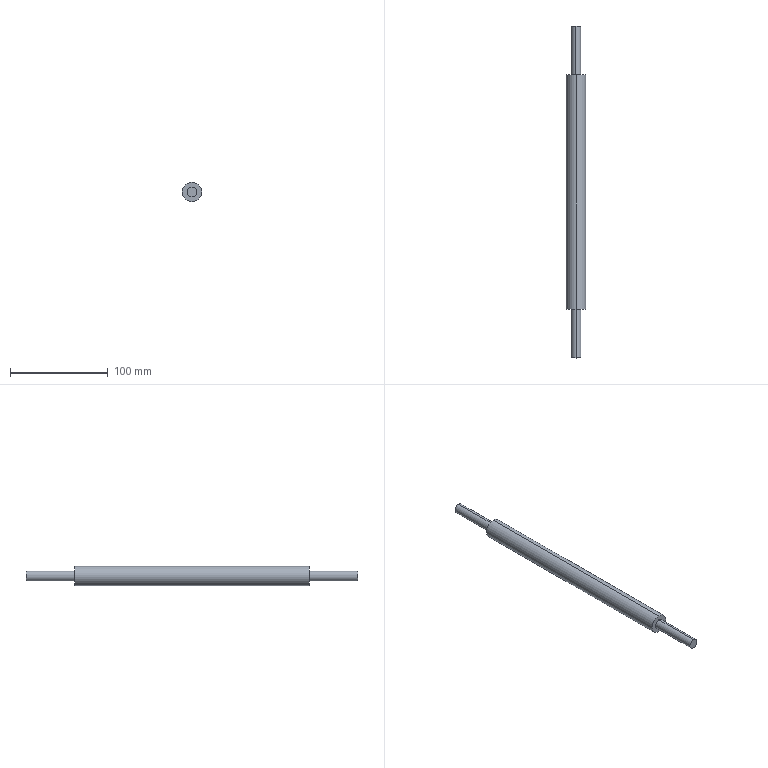Part | STEP file | Fixed long shaft | 1 solid | 10 faces | box 19.77 x 340 x 19.77 mm | volume 81528 mm3 | cylinder 6 | plane 4 | commonest cylinder face diameters 10 x4 19.77 x2
STEP:
#1=CARTESIAN_POINT('',(0.,0.,0.));
#2=DIRECTION('',(0.,0.,1.));
#3=DIRECTION('',(1.,0.,0.));
#4=AXIS2_PLACEMENT_3D('',#1,#2,#3);
#5=CARTESIAN_POINT('',(-0.1215,290.,4.978));
#6=VERTEX_POINT('',#5);
#7=CARTESIAN_POINT('',(-0.1215,290.,-5.022));
#8=VERTEX_POINT('',#7);
#9=CARTESIAN_POINT('',(-0.1215,290.,-0.0221));
#10=DIRECTION('',(0.,1.,0.));
#11=DIRECTION('',(0.,0.,1.));
#12=AXIS2_PLACEMENT_3D('',#9,#10,#11);
#13=CIRCLE('',#12,5.);
#14=CARTESIAN_POINT('',(-0.1215,290.,-0.0221));
#15=DIRECTION('',(0.,-1.,0.));
#16=DIRECTION('',(0.,0.,-1.));
#17=AXIS2_PLACEMENT_3D('',#14,#15,#16);
#18=CYLINDRICAL_SURFACE('',#17,5.);
#19=CARTESIAN_POINT('',(3.142,0.));
#20=DIRECTION('',(-1.,0.));
#21=VECTOR('',#20,1.);
#22=LINE('',#19,#21);
#23=(GEOMETRIC_REPRESENTATION_CONTEXT(2)PARAMETRIC_REPRESENTATION_CONTEXT()REPRESENTATION_CONTEXT('',''));
#24=DEFINITIONAL_REPRESENTATION('',(#22),#23);
#25=PCURVE('',#18,#24);
#26=CARTESIAN_POINT('',(-0.1215,290.,-0.0221));
#27=DIRECTION('',(0.,1.,0.));
#28=DIRECTION('',(0.,0.,1.));
#29=AXIS2_PLACEMENT_3D('',#26,#27,#28);
#30=PLANE('',#29);
#31=CARTESIAN_POINT('',(0.,0.));
#32=DIRECTION('',(1.,0.));
#33=AXIS2_PLACEMENT_2D('',#31,#32);
#34=CIRCLE('',#33,5.);
#35=(GEOMETRIC_REPRESENTATION_CONTEXT(2)PARAMETRIC_REPRESENTATION_CONTEXT()REPRESENTATION_CONTEXT('',''));
#36=DEFINITIONAL_REPRESENTATION('',(#34),#35);
#37=PCURVE('',#30,#36);
#38=SURFACE_CURVE('',#13,(#25,#37),.PCURVE_S1.);
#39=EDGE_CURVE('',#6,#8,#38,.T.);
#40=ORIENTED_EDGE('',*,*,#39,.F.);
#41=CARTESIAN_POINT('',(-0.1215,240.,4.978));
#42=VERTEX_POINT('',#41);
#43=CARTESIAN_POINT('',(-0.1215,290.,4.978));
#44=DIRECTION('',(0.,-1.,0.));
#45=VECTOR('',#44,1.);
#46=LINE('',#43,#45);
#47=CARTESIAN_POINT('',(3.142,0.));
#48=DIRECTION('',(0.,1.));
#49=VECTOR('',#48,1.);
#50=LINE('',#47,#49);
#51=(GEOMETRIC_REPRESENTATION_CONTEXT(2)PARAMETRIC_REPRESENTATION_CONTEXT()REPRESENTATION_CONTEXT('',''));
#52=DEFINITIONAL_REPRESENTATION('',(#50),#51);
#53=PCURVE('',#18,#52);
#54=CARTESIAN_POINT('',(-0.1215,290.,-0.0221));
#55=DIRECTION('',(0.,-1.,0.));
#56=DIRECTION('',(0.,0.,-1.));
#57=AXIS2_PLACEMENT_3D('',#54,#55,#56);
#58=CYLINDRICAL_SURFACE('',#57,5.);
#59=CARTESIAN_POINT('',(3.142,0.));
#60=DIRECTION('',(0.,1.));
#61=VECTOR('',#60,1.);
#62=LINE('',#59,#61);
#63=(GEOMETRIC_REPRESENTATION_CONTEXT(2)PARAMETRIC_REPRESENTATION_CONTEXT()REPRESENTATION_CONTEXT('',''));
#64=DEFINITIONAL_REPRESENTATION('',(#62),#63);
#65=PCURVE('',#58,#64);
#66=SURFACE_CURVE('',#46,(#53,#65),.PCURVE_S1.);
#67=EDGE_CURVE('',#6,#42,#66,.T.);
#68=ORIENTED_EDGE('',*,*,#67,.T.);
#69=CARTESIAN_POINT('',(-0.1215,240.,-5.022));
#70=VERTEX_POINT('',#69);
#71=CARTESIAN_POINT('',(-0.1215,240.,-0.0221));
#72=DIRECTION('',(0.,1.,0.));
#73=DIRECTION('',(0.,0.,1.));
#74=AXIS2_PLACEMENT_3D('',#71,#72,#73);
#75=CIRCLE('',#74,5.);
#76=CARTESIAN_POINT('',(3.142,50.));
#77=DIRECTION('',(-1.,0.));
#78=VECTOR('',#77,1.);
#79=LINE('',#76,#78);
#80=(GEOMETRIC_REPRESENTATION_CONTEXT(2)PARAMETRIC_REPRESENTATION_CONTEXT()REPRESENTATION_CONTEXT('',''));
#81=DEFINITIONAL_REPRESENTATION('',(#79),#80);
#82=PCURVE('',#18,#81);
#83=CARTESIAN_POINT('',(0.,240.,0.));
#84=DIRECTION('',(0.,1.,0.));
#85=DIRECTION('',(0.,0.,1.));
#86=AXIS2_PLACEMENT_3D('',#83,#84,#85);
#87=PLANE('',#86);
#88=CARTESIAN_POINT('',(-0.0221,-0.1215));
#89=DIRECTION('',(1.,0.));
#90=AXIS2_PLACEMENT_2D('',#88,#89);
#91=CIRCLE('',#90,5.);
#92=(GEOMETRIC_REPRESENTATION_CONTEXT(2)PARAMETRIC_REPRESENTATION_CONTEXT()REPRESENTATION_CONTEXT('',''));
#93=DEFINITIONAL_REPRESENTATION('',(#91),#92);
#94=PCURVE('',#87,#93);
#95=SURFACE_CURVE('',#75,(#82,#94),.PCURVE_S1.);
#96=EDGE_CURVE('',#42,#70,#95,.T.);
#97=ORIENTED_EDGE('',*,*,#96,.T.);
#98=CARTESIAN_POINT('',(-0.1215,290.,-5.022));
#99=DIRECTION('',(0.,-1.,0.));
#100=VECTOR('',#99,1.);
#101=LINE('',#98,#100);
#102=CARTESIAN_POINT('',(0.,0.));
#103=DIRECTION('',(0.,1.));
#104=VECTOR('',#103,1.);
#105=LINE('',#102,#104);
#106=(GEOMETRIC_REPRESENTATION_CONTEXT(2)PARAMETRIC_REPRESENTATION_CONTEXT()REPRESENTATION_CONTEXT('',''));
#107=DEFINITIONAL_REPRESENTATION('',(#105),#106);
#108=PCURVE('',#18,#107);
#109=CARTESIAN_POINT('',(6.283,0.));
#110=DIRECTION('',(0.,1.));
#111=VECTOR('',#110,1.);
#112=LINE('',#109,#111);
#113=(GEOMETRIC_REPRESENTATION_CONTEXT(2)PARAMETRIC_REPRESENTATION_CONTEXT()REPRESENTATION_CONTEXT('',''));
#114=DEFINITIONAL_REPRESENTATION('',(#112),#113);
#115=PCURVE('',#58,#114);
#116=SURFACE_CURVE('',#101,(#108,#115),.PCURVE_S1.);
#117=EDGE_CURVE('',#8,#70,#116,.T.);
#118=ORIENTED_EDGE('',*,*,#117,.F.);
#119=EDGE_LOOP('',(#40,#68,#97,#118));
#120=FACE_BOUND('',#119,.T.);
#121=ADVANCED_FACE('',(#120),#18,.T.);
#122=CARTESIAN_POINT('',(0.003134,-50.,-5.018));
#123=VERTEX_POINT('',#122);
#124=CARTESIAN_POINT('',(0.003134,-50.,4.982));
#125=VERTEX_POINT('',#124);
#126=CARTESIAN_POINT('',(0.003134,-50.,-0.01763));
#127=DIRECTION('',(0.,-1.,0.));
#128=DIRECTION('',(0.,0.,-1.));
#129=AXIS2_PLACEMENT_3D('',#126,#127,#128);
#130=CIRCLE('',#129,5.);
#131=CARTESIAN_POINT('',(0.003134,-50.,-0.01763));
#132=DIRECTION('',(0.,1.,0.));
#133=DIRECTION('',(0.,0.,1.));
#134=AXIS2_PLACEMENT_3D('',#131,#132,#133);
#135=CYLINDRICAL_SURFACE('',#134,5.);
#136=CARTESIAN_POINT('',(3.142,0.));
#137=DIRECTION('',(-1.,0.));
#138=VECTOR('',#137,1.);
#139=LINE('',#136,#138);
#140=(GEOMETRIC_REPRESENTATION_CONTEXT(2)PARAMETRIC_REPRESENTATION_CONTEXT()REPRESENTATION_CONTEXT('',''));
#141=DEFINITIONAL_REPRESENTATION('',(#139),#140);
#142=PCURVE('',#135,#141);
#143=CARTESIAN_POINT('',(0.003134,-50.,-0.01763));
#144=DIRECTION('',(0.,-1.,0.));
#145=DIRECTION('',(0.,0.,-1.));
#146=AXIS2_PLACEMENT_3D('',#143,#144,#145);
#147=PLANE('',#146);
#148=CARTESIAN_POINT('',(0.,0.));
#149=DIRECTION('',(1.,0.));
#150=AXIS2_PLACEMENT_2D('',#148,#149);
#151=CIRCLE('',#150,5.);
#152=(GEOMETRIC_REPRESENTATION_CONTEXT(2)PARAMETRIC_REPRESENTATION_CONTEXT()REPRESENTATION_CONTEXT('',''));
#153=DEFINITIONAL_REPRESENTATION('',(#151),#152);
#154=PCURVE('',#147,#153);
#155=SURFACE_CURVE('',#130,(#142,#154),.PCURVE_S1.);
#156=EDGE_CURVE('',#123,#125,#155,.T.);
#157=ORIENTED_EDGE('',*,*,#156,.F.);
#158=CARTESIAN_POINT('',(0.003134,0.,-5.018));
#159=VERTEX_POINT('',#158);
#160=CARTESIAN_POINT('',(0.003134,-50.,-5.018));
#161=DIRECTION('',(0.,1.,0.));
#162=VECTOR('',#161,1.);
#163=LINE('',#160,#162);
#164=CARTESIAN_POINT('',(3.142,0.));
#165=DIRECTION('',(0.,1.));
#166=VECTOR('',#165,1.);
#167=LINE('',#164,#166);
#168=(GEOMETRIC_REPRESENTATION_CONTEXT(2)PARAMETRIC_REPRESENTATION_CONTEXT()REPRESENTATION_CONTEXT('',''));
#169=DEFINITIONAL_REPRESENTATION('',(#167),#168);
#170=PCURVE('',#135,#169);
#171=CARTESIAN_POINT('',(0.003134,-50.,-0.01763));
#172=DIRECTION('',(0.,1.,0.));
#173=DIRECTION('',(0.,0.,1.));
#174=AXIS2_PLACEMENT_3D('',#171,#172,#173);
#175=CYLINDRICAL_SURFACE('',#174,5.);
#176=CARTESIAN_POINT('',(3.142,0.));
#177=DIRECTION('',(0.,1.));
#178=VECTOR('',#177,1.);
#179=LINE('',#176,#178);
#180=(GEOMETRIC_REPRESENTATION_CONTEXT(2)PARAMETRIC_REPRESENTATION_CONTEXT()REPRESENTATION_CONTEXT('',''));
#181=DEFINITIONAL_REPRESENTATION('',(#179),#180);
#182=PCURVE('',#175,#181);
#183=SURFACE_CURVE('',#163,(#170,#182),.PCURVE_S1.);
#184=EDGE_CURVE('',#123,#159,#183,.T.);
#185=ORIENTED_EDGE('',*,*,#184,.T.);
#186=CARTESIAN_POINT('',(0.003134,0.,4.982));
#187=VERTEX_POINT('',#186);
#188=CARTESIAN_POINT('',(0.003134,0.,-0.01763));
#189=DIRECTION('',(0.,-1.,0.));
#190=DIRECTION('',(0.,0.,-1.));
#191=AXIS2_PLACEMENT_3D('',#188,#189,#190);
#192=CIRCLE('',#191,5.);
#193=CARTESIAN_POINT('',(3.142,50.));
#194=DIRECTION('',(-1.,0.));
#195=VECTOR('',#194,1.);
#196=LINE('',#193,#195);
#197=(GEOMETRIC_REPRESENTATION_CONTEXT(2)PARAMETRIC_REPRESENTATION_CONTEXT()REPRESENTATION_CONTEXT('',''));
#198=DEFINITIONAL_REPRESENTATION('',(#196),#197);
#199=PCURVE('',#135,#198);
#200=CARTESIAN_POINT('',(0.,0.,0.));
#201=DIRECTION('',(0.,1.,0.));
#202=DIRECTION('',(0.,0.,1.));
#203=AXIS2_PLACEMENT_3D('',#200,#201,#202);
#204=PLANE('',#203);
#205=CARTESIAN_POINT('',(-5.018,0.003134));
#206=CARTESIAN_POINT('',(-5.018,8.663));
#207=CARTESIAN_POINT('',(2.482,4.333));
#208=CARTESIAN_POINT('',(9.982,0.003134));
#209=CARTESIAN_POINT('',(2.482,-4.327));
#210=CARTESIAN_POINT('',(-5.018,-8.657));
#211=CARTESIAN_POINT('',(-5.018,0.003134));
#212=(BOUNDED_CURVE()B_SPLINE_CURVE(2,(#205,#206,#207,#208,#209,#210,#211),.UNSPECIFIED.,.T.,.F.)B_SPLINE_CURVE_WITH_KNOTS((1,2,2,2,2,1),(-2.094,0.,2.094,4.189,6.283,8.378),.UNSPECIFIED.)CURVE()GEOMETRIC_REPRESENTATION_ITEM()RATIONAL_B_SPLINE_CURVE((1.,0.5,1.,0.5,1.,0.5,1.))REPRESENTATION_ITEM(''));
#213=(GEOMETRIC_REPRESENTATION_CONTEXT(2)PARAMETRIC_REPRESENTATION_CONTEXT()REPRESENTATION_CONTEXT('',''));
#214=DEFINITIONAL_REPRESENTATION('',(#212),#213);
#215=PCURVE('',#204,#214);
#216=SURFACE_CURVE('',#192,(#199,#215),.PCURVE_S1.);
#217=EDGE_CURVE('',#159,#187,#216,.T.);
#218=ORIENTED_EDGE('',*,*,#217,.T.);
#219=CARTESIAN_POINT('',(0.003134,-50.,4.982));
#220=DIRECTION('',(0.,1.,0.));
#221=VECTOR('',#220,1.);
#222=LINE('',#219,#221);
#223=CARTESIAN_POINT('',(0.,0.));
#224=DIRECTION('',(0.,1.));
#225=VECTOR('',#224,1.);
#226=LINE('',#223,#225);
#227=(GEOMETRIC_REPRESENTATION_CONTEXT(2)PARAMETRIC_REPRESENTATION_CONTEXT()REPRESENTATION_CONTEXT('',''));
#228=DEFINITIONAL_REPRESENTATION('',(#226),#227);
#229=PCURVE('',#135,#228);
#230=CARTESIAN_POINT('',(6.283,0.));
#231=DIRECTION('',(0.,1.));
#232=VECTOR('',#231,1.);
#233=LINE('',#230,#232);
#234=(GEOMETRIC_REPRESENTATION_CONTEXT(2)PARAMETRIC_REPRESENTATION_CONTEXT()REPRESENTATION_CONTEXT('',''));
#235=DEFINITIONAL_REPRESENTATION('',(#233),#234);
#236=PCURVE('',#175,#235);
#237=SURFACE_CURVE('',#222,(#229,#236),.PCURVE_S1.);
#238=EDGE_CURVE('',#125,#187,#237,.T.);
#239=ORIENTED_EDGE('',*,*,#238,.F.);
#240=EDGE_LOOP('',(#157,#185,#218,#239));
#241=FACE_BOUND('',#240,.T.);
#242=ADVANCED_FACE('',(#241),#135,.T.);
#243=CARTESIAN_POINT('',(0.,240.,9.885));
#244=VERTEX_POINT('',#243);
#245=CARTESIAN_POINT('',(0.,240.,-9.885));
#246=VERTEX_POINT('',#245);
#247=CARTESIAN_POINT('',(0.,240.,0.));
#248=DIRECTION('',(0.,1.,0.));
#249=DIRECTION('',(0.,0.,1.));
#250=AXIS2_PLACEMENT_3D('',#247,#248,#249);
#251=CIRCLE('',#250,9.885);
#252=CARTESIAN_POINT('',(0.,240.,0.));
#253=DIRECTION('',(0.,-1.,0.));
#254=DIRECTION('',(0.,0.,-1.));
#255=AXIS2_PLACEMENT_3D('',#252,#253,#254);
#256=CYLINDRICAL_SURFACE('',#255,9.885);
#257=CARTESIAN_POINT('',(3.142,0.));
#258=DIRECTION('',(-1.,0.));
#259=VECTOR('',#258,1.);
#260=LINE('',#257,#259);
#261=(GEOMETRIC_REPRESENTATION_CONTEXT(2)PARAMETRIC_REPRESENTATION_CONTEXT()REPRESENTATION_CONTEXT('',''));
#262=DEFINITIONAL_REPRESENTATION('',(#260),#261);
#263=PCURVE('',#256,#262);
#264=CARTESIAN_POINT('',(0.,0.));
#265=DIRECTION('',(1.,0.));
#266=AXIS2_PLACEMENT_2D('',#264,#265);
#267=CIRCLE('',#266,9.885);
#268=(GEOMETRIC_REPRESENTATION_CONTEXT(2)PARAMETRIC_REPRESENTATION_CONTEXT()REPRESENTATION_CONTEXT('',''));
#269=DEFINITIONAL_REPRESENTATION('',(#267),#268);
#270=PCURVE('',#87,#269);
#271=SURFACE_CURVE('',#251,(#263,#270),.PCURVE_S1.);
#272=EDGE_CURVE('',#244,#246,#271,.T.);
#273=ORIENTED_EDGE('',*,*,#272,.F.);
#274=CARTESIAN_POINT('',(0.,0.,9.885));
#275=VERTEX_POINT('',#274);
#276=CARTESIAN_POINT('',(0.,240.,9.885));
#277=DIRECTION('',(0.,-1.,0.));
#278=VECTOR('',#277,1.);
#279=LINE('',#276,#278);
#280=CARTESIAN_POINT('',(3.142,0.));
#281=DIRECTION('',(0.,1.));
#282=VECTOR('',#281,1.);
#283=LINE('',#280,#282);
#284=(GEOMETRIC_REPRESENTATION_CONTEXT(2)PARAMETRIC_REPRESENTATION_CONTEXT()REPRESENTATION_CONTEXT('',''));
#285=DEFINITIONAL_REPRESENTATION('',(#283),#284);
#286=PCURVE('',#256,#285);
#287=CARTESIAN_POINT('',(0.,240.,0.));
#288=DIRECTION('',(0.,-1.,0.));
#289=DIRECTION('',(0.,0.,-1.));
#290=AXIS2_PLACEMENT_3D('',#287,#288,#289);
#291=CYLINDRICAL_SURFACE('',#290,9.885);
#292=CARTESIAN_POINT('',(3.142,0.));
#293=DIRECTION('',(0.,1.));
#294=VECTOR('',#293,1.);
#295=LINE('',#292,#294);
#296=(GEOMETRIC_REPRESENTATION_CONTEXT(2)PARAMETRIC_REPRESENTATION_CONTEXT()REPRESENTATION_CONTEXT('',''));
#297=DEFINITIONAL_REPRESENTATION('',(#295),#296);
#298=PCURVE('',#291,#297);
#299=SURFACE_CURVE('',#279,(#286,#298),.PCURVE_S1.);
#300=EDGE_CURVE('',#244,#275,#299,.T.);
#301=ORIENTED_EDGE('',*,*,#300,.T.);
#302=CARTESIAN_POINT('',(0.,0.,-9.885));
#303=VERTEX_POINT('',#302);
#304=CARTESIAN_POINT('',(0.,0.,0.));
#305=DIRECTION('',(0.,1.,0.));
#306=DIRECTION('',(0.,0.,1.));
#307=AXIS2_PLACEMENT_3D('',#304,#305,#306);
#308=CIRCLE('',#307,9.885);
#309=CARTESIAN_POINT('',(3.142,240.));
#310=DIRECTION('',(-1.,0.));
#311=VECTOR('',#310,1.);
#312=LINE('',#309,#311);
#313=(GEOMETRIC_REPRESENTATION_CONTEXT(2)PARAMETRIC_REPRESENTATION_CONTEXT()REPRESENTATION_CONTEXT('',''));
#314=DEFINITIONAL_REPRESENTATION('',(#312),#313);
#315=PCURVE('',#256,#314);
#316=CARTESIAN_POINT('',(0.,0.));
#317=DIRECTION('',(1.,0.));
#318=AXIS2_PLACEMENT_2D('',#316,#317);
#319=CIRCLE('',#318,9.885);
#320=(GEOMETRIC_REPRESENTATION_CONTEXT(2)PARAMETRIC_REPRESENTATION_CONTEXT()REPRESENTATION_CONTEXT('',''));
#321=DEFINITIONAL_REPRESENTATION('',(#319),#320);
#322=PCURVE('',#204,#321);
#323=SURFACE_CURVE('',#308,(#315,#322),.PCURVE_S1.);
#324=EDGE_CURVE('',#275,#303,#323,.T.);
#325=ORIENTED_EDGE('',*,*,#324,.T.);
#326=CARTESIAN_POINT('',(0.,240.,-9.885));
#327=DIRECTION('',(0.,-1.,0.));
#328=VECTOR('',#327,1.);
#329=LINE('',#326,#328);
#330=CARTESIAN_POINT('',(0.,0.));
#331=DIRECTION('',(0.,1.));
#332=VECTOR('',#331,1.);
#333=LINE('',#330,#332);
#334=(GEOMETRIC_REPRESENTATION_CONTEXT(2)PARAMETRIC_REPRESENTATION_CONTEXT()REPRESENTATION_CONTEXT('',''));
#335=DEFINITIONAL_REPRESENTATION('',(#333),#334);
#336=PCURVE('',#256,#335);
#337=CARTESIAN_POINT('',(6.283,0.));
#338=DIRECTION('',(0.,1.));
#339=VECTOR('',#338,1.);
#340=LINE('',#337,#339);
#341=(GEOMETRIC_REPRESENTATION_CONTEXT(2)PARAMETRIC_REPRESENTATION_CONTEXT()REPRESENTATION_CONTEXT('',''));
#342=DEFINITIONAL_REPRESENTATION('',(#340),#341);
#343=PCURVE('',#291,#342);
#344=SURFACE_CURVE('',#329,(#336,#343),.PCURVE_S1.);
#345=EDGE_CURVE('',#246,#303,#344,.T.);
#346=ORIENTED_EDGE('',*,*,#345,.F.);
#347=EDGE_LOOP('',(#273,#301,#325,#346));
#348=FACE_BOUND('',#347,.T.);
#349=ADVANCED_FACE('',(#348),#256,.T.);
#350=ORIENTED_EDGE('',*,*,#300,.F.);
#351=CARTESIAN_POINT('',(0.,240.,0.));
#352=DIRECTION('',(0.,1.,0.));
#353=DIRECTION('',(0.,0.,1.));
#354=AXIS2_PLACEMENT_3D('',#351,#352,#353);
#355=CIRCLE('',#354,9.885);
#356=CARTESIAN_POINT('',(9.425,0.));
#357=DIRECTION('',(-1.,0.));
#358=VECTOR('',#357,1.);
#359=LINE('',#356,#358);
#360=(GEOMETRIC_REPRESENTATION_CONTEXT(2)PARAMETRIC_REPRESENTATION_CONTEXT()REPRESENTATION_CONTEXT('',''));
#361=DEFINITIONAL_REPRESENTATION('',(#359),#360);
#362=PCURVE('',#291,#361);
#363=CARTESIAN_POINT('',(0.,0.));
#364=DIRECTION('',(1.,0.));
#365=AXIS2_PLACEMENT_2D('',#363,#364);
#366=CIRCLE('',#365,9.885);
#367=(GEOMETRIC_REPRESENTATION_CONTEXT(2)PARAMETRIC_REPRESENTATION_CONTEXT()REPRESENTATION_CONTEXT('',''));
#368=DEFINITIONAL_REPRESENTATION('',(#366),#367);
#369=PCURVE('',#87,#368);
#370=SURFACE_CURVE('',#355,(#362,#369),.PCURVE_S1.);
#371=EDGE_CURVE('',#246,#244,#370,.T.);
#372=ORIENTED_EDGE('',*,*,#371,.F.);
#373=ORIENTED_EDGE('',*,*,#345,.T.);
#374=CARTESIAN_POINT('',(0.,0.,0.));
#375=DIRECTION('',(0.,1.,0.));
#376=DIRECTION('',(0.,0.,1.));
#377=AXIS2_PLACEMENT_3D('',#374,#375,#376);
#378=CIRCLE('',#377,9.885);
#379=CARTESIAN_POINT('',(9.425,240.));
#380=DIRECTION('',(-1.,0.));
#381=VECTOR('',#380,1.);
#382=LINE('',#379,#381);
#383=(GEOMETRIC_REPRESENTATION_CONTEXT(2)PARAMETRIC_REPRESENTATION_CONTEXT()REPRESENTATION_CONTEXT('',''));
#384=DEFINITIONAL_REPRESENTATION('',(#382),#383);
#385=PCURVE('',#291,#384);
#386=CARTESIAN_POINT('',(0.,0.));
#387=DIRECTION('',(1.,0.));
#388=AXIS2_PLACEMENT_2D('',#386,#387);
#389=CIRCLE('',#388,9.885);
#390=(GEOMETRIC_REPRESENTATION_CONTEXT(2)PARAMETRIC_REPRESENTATION_CONTEXT()REPRESENTATION_CONTEXT('',''));
#391=DEFINITIONAL_REPRESENTATION('',(#389),#390);
#392=PCURVE('',#204,#391);
#393=SURFACE_CURVE('',#378,(#385,#392),.PCURVE_S1.);
#394=EDGE_CURVE('',#303,#275,#393,.T.);
#395=ORIENTED_EDGE('',*,*,#394,.T.);
#396=EDGE_LOOP('',(#350,#372,#373,#395));
#397=FACE_BOUND('',#396,.T.);
#398=ADVANCED_FACE('',(#397),#291,.T.);
#399=CARTESIAN_POINT('',(-0.1215,240.,-0.0221));
#400=DIRECTION('',(0.,1.,0.));
#401=DIRECTION('',(0.,0.,1.));
#402=AXIS2_PLACEMENT_3D('',#399,#400,#401);
#403=CIRCLE('',#402,5.);
#404=CARTESIAN_POINT('',(-0.0221,-0.1215));
#405=DIRECTION('',(1.,0.));
#406=AXIS2_PLACEMENT_2D('',#404,#405);
#407=CIRCLE('',#406,5.);
#408=(GEOMETRIC_REPRESENTATION_CONTEXT(2)PARAMETRIC_REPRESENTATION_CONTEXT()REPRESENTATION_CONTEXT('',''));
#409=DEFINITIONAL_REPRESENTATION('',(#407),#408);
#410=PCURVE('',#87,#409);
#411=CARTESIAN_POINT('',(9.425,50.));
#412=DIRECTION('',(-1.,0.));
#413=VECTOR('',#412,1.);
#414=LINE('',#411,#413);
#415=(GEOMETRIC_REPRESENTATION_CONTEXT(2)PARAMETRIC_REPRESENTATION_CONTEXT()REPRESENTATION_CONTEXT('',''));
#416=DEFINITIONAL_REPRESENTATION('',(#414),#415);
#417=PCURVE('',#58,#416);
#418=SURFACE_CURVE('',#403,(#410,#417),.PCURVE_S1.);
#419=EDGE_CURVE('',#70,#42,#418,.T.);
#420=ORIENTED_EDGE('',*,*,#419,.F.);
#421=ORIENTED_EDGE('',*,*,#96,.F.);
#422=EDGE_LOOP('',(#420,#421));
#423=FACE_BOUND('',#422,.T.);
#424=ORIENTED_EDGE('',*,*,#371,.T.);
#425=ORIENTED_EDGE('',*,*,#272,.T.);
#426=EDGE_LOOP('',(#424,#425));
#427=FACE_BOUND('',#426,.T.);
#428=ADVANCED_FACE('',(#423,#427),#87,.T.);
#429=CARTESIAN_POINT('',(0.003134,0.,-0.01763));
#430=DIRECTION('',(0.,-1.,0.));
#431=DIRECTION('',(0.,0.,-1.));
#432=AXIS2_PLACEMENT_3D('',#429,#430,#431);
#433=CIRCLE('',#432,5.);
#434=CARTESIAN_POINT('',(-5.018,0.003134));
#435=CARTESIAN_POINT('',(-5.018,8.663));
#436=CARTESIAN_POINT('',(2.482,4.333));
#437=CARTESIAN_POINT('',(9.982,0.003134));
#438=CARTESIAN_POINT('',(2.482,-4.327));
#439=CARTESIAN_POINT('',(-5.018,-8.657));
#440=CARTESIAN_POINT('',(-5.018,0.003134));
#441=(BOUNDED_CURVE()B_SPLINE_CURVE(2,(#434,#435,#436,#437,#438,#439,#440),.UNSPECIFIED.,.T.,.F.)B_SPLINE_CURVE_WITH_KNOTS((1,2,2,2,2,1),(-2.094,0.,2.094,4.189,6.283,8.378),.UNSPECIFIED.)CURVE()GEOMETRIC_REPRESENTATION_ITEM()RATIONAL_B_SPLINE_CURVE((1.,0.5,1.,0.5,1.,0.5,1.))REPRESENTATION_ITEM(''));
#442=(GEOMETRIC_REPRESENTATION_CONTEXT(2)PARAMETRIC_REPRESENTATION_CONTEXT()REPRESENTATION_CONTEXT('',''));
#443=DEFINITIONAL_REPRESENTATION('',(#441),#442);
#444=PCURVE('',#204,#443);
#445=CARTESIAN_POINT('',(9.425,50.));
#446=DIRECTION('',(-1.,0.));
#447=VECTOR('',#446,1.);
#448=LINE('',#445,#447);
#449=(GEOMETRIC_REPRESENTATION_CONTEXT(2)PARAMETRIC_REPRESENTATION_CONTEXT()REPRESENTATION_CONTEXT('',''));
#450=DEFINITIONAL_REPRESENTATION('',(#448),#449);
#451=PCURVE('',#175,#450);
#452=SURFACE_CURVE('',#433,(#444,#451),.PCURVE_S1.);
#453=EDGE_CURVE('',#187,#159,#452,.T.);
#454=ORIENTED_EDGE('',*,*,#453,.F.);
#455=ORIENTED_EDGE('',*,*,#217,.F.);
#456=EDGE_LOOP('',(#454,#455));
#457=FACE_BOUND('',#456,.T.);
#458=ORIENTED_EDGE('',*,*,#394,.F.);
#459=ORIENTED_EDGE('',*,*,#324,.F.);
#460=EDGE_LOOP('',(#458,#459));
#461=FACE_BOUND('',#460,.T.);
#462=ADVANCED_FACE('',(#457,#461),#204,.F.);
#463=ORIENTED_EDGE('',*,*,#184,.F.);
#464=CARTESIAN_POINT('',(0.003134,-50.,-0.01763));
#465=DIRECTION('',(0.,-1.,0.));
#466=DIRECTION('',(0.,0.,-1.));
#467=AXIS2_PLACEMENT_3D('',#464,#465,#466);
#468=CIRCLE('',#467,5.);
#469=CARTESIAN_POINT('',(9.425,0.));
#470=DIRECTION('',(-1.,0.));
#471=VECTOR('',#470,1.);
#472=LINE('',#469,#471);
#473=(GEOMETRIC_REPRESENTATION_CONTEXT(2)PARAMETRIC_REPRESENTATION_CONTEXT()REPRESENTATION_CONTEXT('',''));
#474=DEFINITIONAL_REPRESENTATION('',(#472),#473);
#475=PCURVE('',#175,#474);
#476=CARTESIAN_POINT('',(0.,0.));
#477=DIRECTION('',(1.,0.));
#478=AXIS2_PLACEMENT_2D('',#476,#477);
#479=CIRCLE('',#478,5.);
#480=(GEOMETRIC_REPRESENTATION_CONTEXT(2)PARAMETRIC_REPRESENTATION_CONTEXT()REPRESENTATION_CONTEXT('',''));
#481=DEFINITIONAL_REPRESENTATION('',(#479),#480);
#482=PCURVE('',#147,#481);
#483=SURFACE_CURVE('',#468,(#475,#482),.PCURVE_S1.);
#484=EDGE_CURVE('',#125,#123,#483,.T.);
#485=ORIENTED_EDGE('',*,*,#484,.F.);
#486=ORIENTED_EDGE('',*,*,#238,.T.);
#487=ORIENTED_EDGE('',*,*,#453,.T.);
#488=EDGE_LOOP('',(#463,#485,#486,#487));
#489=FACE_BOUND('',#488,.T.);
#490=ADVANCED_FACE('',(#489),#175,.T.);
#491=ORIENTED_EDGE('',*,*,#484,.T.);
#492=ORIENTED_EDGE('',*,*,#156,.T.);
#493=EDGE_LOOP('',(#491,#492));
#494=FACE_BOUND('',#493,.T.);
#495=ADVANCED_FACE('',(#494),#147,.T.);
#496=ORIENTED_EDGE('',*,*,#67,.F.);
#497=CARTESIAN_POINT('',(-0.1215,290.,-0.0221));
#498=DIRECTION('',(0.,1.,0.));
#499=DIRECTION('',(0.,0.,1.));
#500=AXIS2_PLACEMENT_3D('',#497,#498,#499);
#501=CIRCLE('',#500,5.);
#502=CARTESIAN_POINT('',(9.425,0.));
#503=DIRECTION('',(-1.,0.));
#504=VECTOR('',#503,1.);
#505=LINE('',#502,#504);
#506=(GEOMETRIC_REPRESENTATION_CONTEXT(2)PARAMETRIC_REPRESENTATION_CONTEXT()REPRESENTATION_CONTEXT('',''));
#507=DEFINITIONAL_REPRESENTATION('',(#505),#506);
#508=PCURVE('',#58,#507);
#509=CARTESIAN_POINT('',(0.,0.));
#510=DIRECTION('',(1.,0.));
#511=AXIS2_PLACEMENT_2D('',#509,#510);
#512=CIRCLE('',#511,5.);
#513=(GEOMETRIC_REPRESENTATION_CONTEXT(2)PARAMETRIC_REPRESENTATION_CONTEXT()REPRESENTATION_CONTEXT('',''));
#514=DEFINITIONAL_REPRESENTATION('',(#512),#513);
#515=PCURVE('',#30,#514);
#516=SURFACE_CURVE('',#501,(#508,#515),.PCURVE_S1.);
#517=EDGE_CURVE('',#8,#6,#516,.T.);
#518=ORIENTED_EDGE('',*,*,#517,.F.);
#519=ORIENTED_EDGE('',*,*,#117,.T.);
#520=ORIENTED_EDGE('',*,*,#419,.T.);
#521=EDGE_LOOP('',(#496,#518,#519,#520));
#522=FACE_BOUND('',#521,.T.);
#523=ADVANCED_FACE('',(#522),#58,.T.);
#524=ORIENTED_EDGE('',*,*,#517,.T.);
#525=ORIENTED_EDGE('',*,*,#39,.T.);
#526=EDGE_LOOP('',(#524,#525));
#527=FACE_BOUND('',#526,.T.);
#528=ADVANCED_FACE('',(#527),#30,.T.);
#529=CLOSED_SHELL('',(#121,#242,#349,#398,#428,#462,#490,#495,#523,#528));
#530=MANIFOLD_SOLID_BREP('',#529);
#531=(LENGTH_UNIT()NAMED_UNIT(*)SI_UNIT(.MILLI.,.METRE.));
#532=UNCERTAINTY_MEASURE_WITH_UNIT(LENGTH_MEASURE(0.0000001),#531,'','');
#533=(NAMED_UNIT(*)PLANE_ANGLE_UNIT()SI_UNIT($,.RADIAN.));
#534=(NAMED_UNIT(*)SI_UNIT($,.STERADIAN.)SOLID_ANGLE_UNIT());
#535=(GEOMETRIC_REPRESENTATION_CONTEXT(3)GLOBAL_UNCERTAINTY_ASSIGNED_CONTEXT((#532))GLOBAL_UNIT_ASSIGNED_CONTEXT((#531,#533,#534))REPRESENTATION_CONTEXT('',''));
#536=ADVANCED_BREP_SHAPE_REPRESENTATION('',(#4,#530),#535);